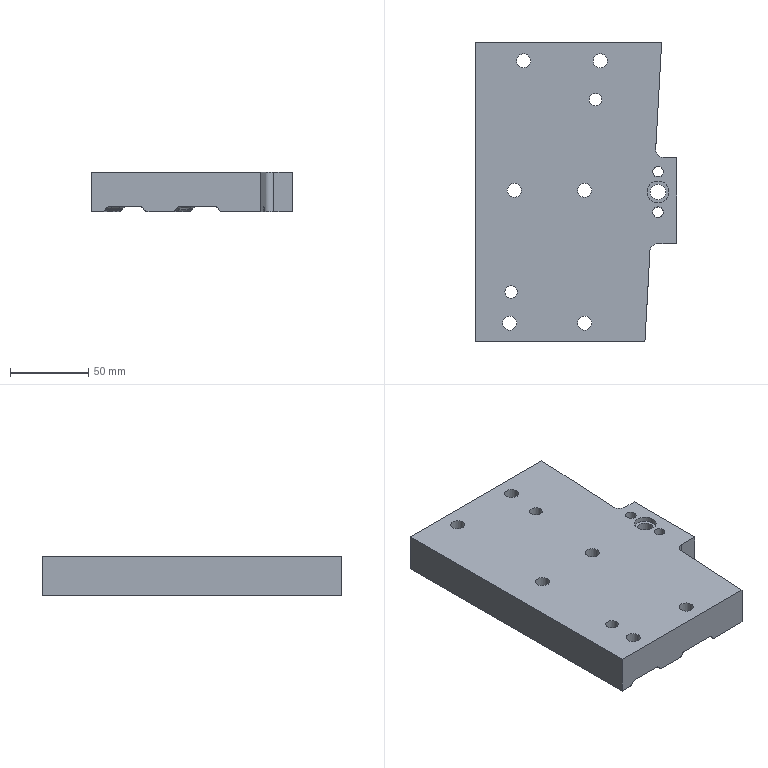Part | NX | features solid 2 | 1 solid | 128 faces | box 129 x 192 x 25 mm | volume 506496 mm3 | cylinder 60 | plane 28 | torus 26 | spline 14 | commonest cylinder face diameters 4 x19 5 x11 9 x6 14.5 x6 3 x4 6 x4